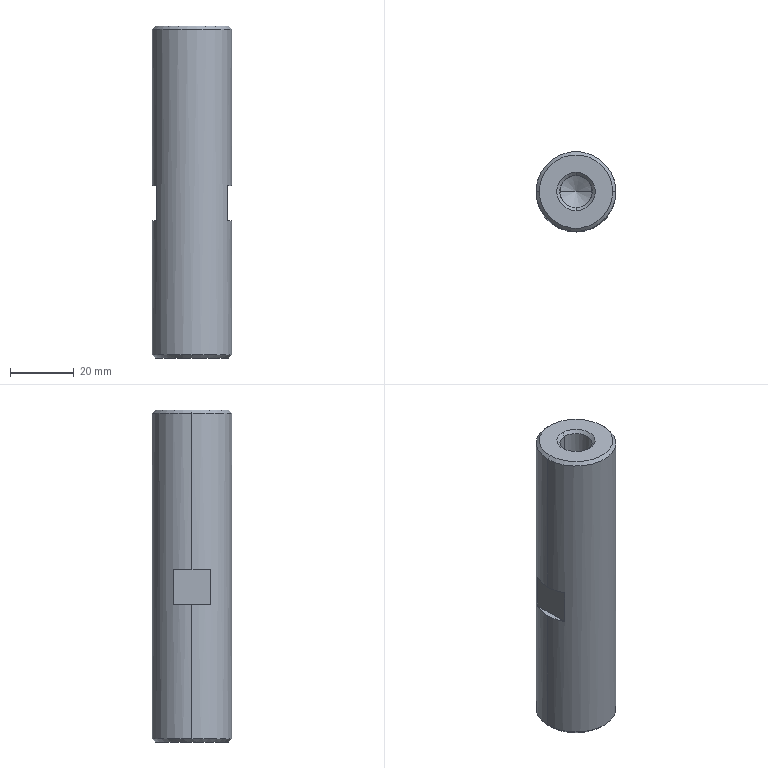Part | SolidWorks | features BaseBody 1, MoveFace 1 | 1 solid | 26 faces | box 25 x 25 x 104 mm | volume 46673 mm3 | cone 12 | plane 8 | cylinder 6 | commonest cylinder face diameters 10.106 x4 25 x2
STEP:
#1=CARTESIAN_POINT('',(0.,12.5,-103.));
#2=VERTEX_POINT('',#1);
#3=CARTESIAN_POINT('',(-12.5,0.,-103.));
#4=VERTEX_POINT('',#3);
#5=CARTESIAN_POINT('',(0.,0.,-103.));
#6=DIRECTION('',(0.,0.,1.));
#7=DIRECTION('',(1.,0.,0.));
#8=AXIS2_PLACEMENT_3D('',#5,#6,#7);
#9=CIRCLE('',#8,12.5);
#10=EDGE_CURVE('',#2,#4,#9,.T.);
#11=ORIENTED_EDGE('',*,*,#10,.T.);
#12=CARTESIAN_POINT('',(-12.5,0.,-61.));
#13=VERTEX_POINT('',#12);
#14=CARTESIAN_POINT('',(-12.5,0.,-106.));
#15=DIRECTION('',(0.,0.,1.));
#16=VECTOR('',#15,1000.);
#17=LINE('',#14,#16);
#18=EDGE_CURVE('',#4,#13,#17,.T.);
#19=ORIENTED_EDGE('',*,*,#18,.T.);
#20=CARTESIAN_POINT('',(-11.,5.937,-61.));
#21=VERTEX_POINT('',#20);
#22=CARTESIAN_POINT('',(0.,0.,-61.));
#23=DIRECTION('',(0.,0.,-1.));
#24=DIRECTION('',(1.,0.,0.));
#25=AXIS2_PLACEMENT_3D('',#22,#23,#24);
#26=CIRCLE('',#25,12.5);
#27=EDGE_CURVE('',#13,#21,#26,.T.);
#28=ORIENTED_EDGE('',*,*,#27,.T.);
#29=CARTESIAN_POINT('',(-11.,5.937,-50.));
#30=VERTEX_POINT('',#29);
#31=CARTESIAN_POINT('',(-11.,5.937,-106.));
#32=DIRECTION('',(0.,0.,1.));
#33=VECTOR('',#32,1000.);
#34=LINE('',#31,#33);
#35=EDGE_CURVE('',#21,#30,#34,.T.);
#36=ORIENTED_EDGE('',*,*,#35,.T.);
#37=CARTESIAN_POINT('',(-12.5,0.,-50.));
#38=VERTEX_POINT('',#37);
#39=CARTESIAN_POINT('',(0.,0.,-50.));
#40=DIRECTION('',(0.,0.,1.));
#41=DIRECTION('',(1.,0.,0.));
#42=AXIS2_PLACEMENT_3D('',#39,#40,#41);
#43=CIRCLE('',#42,12.5);
#44=EDGE_CURVE('',#30,#38,#43,.T.);
#45=ORIENTED_EDGE('',*,*,#44,.T.);
#46=CARTESIAN_POINT('',(-12.5,0.,-1.));
#47=VERTEX_POINT('',#46);
#48=CARTESIAN_POINT('',(-12.5,0.,-106.));
#49=DIRECTION('',(0.,0.,1.));
#50=VECTOR('',#49,1000.);
#51=LINE('',#48,#50);
#52=EDGE_CURVE('',#38,#47,#51,.T.);
#53=ORIENTED_EDGE('',*,*,#52,.T.);
#54=CARTESIAN_POINT('',(12.5,0.,-1.));
#55=VERTEX_POINT('',#54);
#56=CARTESIAN_POINT('',(0.,0.,-1.));
#57=DIRECTION('',(0.,0.,-1.));
#58=DIRECTION('',(1.,0.,0.));
#59=AXIS2_PLACEMENT_3D('',#56,#57,#58);
#60=CIRCLE('',#59,12.5);
#61=EDGE_CURVE('',#47,#55,#60,.T.);
#62=ORIENTED_EDGE('',*,*,#61,.T.);
#63=CARTESIAN_POINT('',(12.5,0.,-50.));
#64=VERTEX_POINT('',#63);
#65=CARTESIAN_POINT('',(12.5,0.,-106.));
#66=DIRECTION('',(0.,0.,1.));
#67=VECTOR('',#66,1000.);
#68=LINE('',#65,#67);
#69=EDGE_CURVE('',#64,#55,#68,.T.);
#70=ORIENTED_EDGE('',*,*,#69,.F.);
#71=CARTESIAN_POINT('',(11.,5.937,-50.));
#72=VERTEX_POINT('',#71);
#73=CARTESIAN_POINT('',(0.,0.,-50.));
#74=DIRECTION('',(0.,0.,1.));
#75=DIRECTION('',(1.,0.,0.));
#76=AXIS2_PLACEMENT_3D('',#73,#74,#75);
#77=CIRCLE('',#76,12.5);
#78=EDGE_CURVE('',#64,#72,#77,.T.);
#79=ORIENTED_EDGE('',*,*,#78,.T.);
#80=CARTESIAN_POINT('',(11.,5.937,-61.));
#81=VERTEX_POINT('',#80);
#82=CARTESIAN_POINT('',(11.,5.937,-106.));
#83=DIRECTION('',(0.,0.,-1.));
#84=VECTOR('',#83,1000.);
#85=LINE('',#82,#84);
#86=EDGE_CURVE('',#72,#81,#85,.T.);
#87=ORIENTED_EDGE('',*,*,#86,.T.);
#88=CARTESIAN_POINT('',(12.5,0.,-61.));
#89=VERTEX_POINT('',#88);
#90=CARTESIAN_POINT('',(0.,0.,-61.));
#91=DIRECTION('',(0.,0.,-1.));
#92=DIRECTION('',(1.,0.,0.));
#93=AXIS2_PLACEMENT_3D('',#90,#91,#92);
#94=CIRCLE('',#93,12.5);
#95=EDGE_CURVE('',#81,#89,#94,.T.);
#96=ORIENTED_EDGE('',*,*,#95,.T.);
#97=CARTESIAN_POINT('',(12.5,0.,-103.));
#98=VERTEX_POINT('',#97);
#99=CARTESIAN_POINT('',(12.5,0.,-106.));
#100=DIRECTION('',(0.,0.,1.));
#101=VECTOR('',#100,1000.);
#102=LINE('',#99,#101);
#103=EDGE_CURVE('',#98,#89,#102,.T.);
#104=ORIENTED_EDGE('',*,*,#103,.F.);
#105=CARTESIAN_POINT('',(0.,0.,-103.));
#106=DIRECTION('',(0.,0.,1.));
#107=DIRECTION('',(1.,0.,0.));
#108=AXIS2_PLACEMENT_3D('',#105,#106,#107);
#109=CIRCLE('',#108,12.5);
#110=EDGE_CURVE('',#98,#2,#109,.T.);
#111=ORIENTED_EDGE('',*,*,#110,.T.);
#112=EDGE_LOOP('',(#11,#19,#28,#36,#45,#53,#62,#70,#79,#87,#96,#104,#111));
#113=FACE_OUTER_BOUND('',#112,.T.);
#114=CARTESIAN_POINT('',(0.,0.,-106.));
#115=DIRECTION('',(0.,0.,1.));
#116=DIRECTION('',(1.,0.,0.));
#117=AXIS2_PLACEMENT_3D('',#114,#115,#116);
#118=CYLINDRICAL_SURFACE('',#117,12.5);
#119=ADVANCED_FACE('',(#113),#118,.T.);
#120=CARTESIAN_POINT('',(-11.5,0.,0.));
#121=VERTEX_POINT('',#120);
#122=CARTESIAN_POINT('',(11.5,0.,0.));
#123=VERTEX_POINT('',#122);
#124=CARTESIAN_POINT('',(0.,0.,0.));
#125=DIRECTION('',(0.,0.,-1.));
#126=DIRECTION('',(-1.,0.,0.));
#127=AXIS2_PLACEMENT_3D('',#124,#125,#126);
#128=CIRCLE('',#127,11.5);
#129=EDGE_CURVE('',#121,#123,#128,.T.);
#130=ORIENTED_EDGE('',*,*,#129,.T.);
#131=CARTESIAN_POINT('',(12.5,0.,-1.));
#132=DIRECTION('',(0.7071,0.,-0.7071));
#133=VECTOR('',#132,1000.);
#134=LINE('',#131,#133);
#135=EDGE_CURVE('',#123,#55,#134,.T.);
#136=ORIENTED_EDGE('',*,*,#135,.T.);
#137=ORIENTED_EDGE('',*,*,#61,.F.);
#138=CARTESIAN_POINT('',(-12.5,0.,-1.));
#139=DIRECTION('',(-0.7071,0.,-0.7071));
#140=VECTOR('',#139,1000.);
#141=LINE('',#138,#140);
#142=EDGE_CURVE('',#121,#47,#141,.T.);
#143=ORIENTED_EDGE('',*,*,#142,.F.);
#144=EDGE_LOOP('',(#130,#136,#137,#143));
#145=FACE_OUTER_BOUND('',#144,.T.);
#146=CARTESIAN_POINT('',(0.,0.,-1.));
#147=DIRECTION('',(0.,0.,-1.));
#148=DIRECTION('',(-1.,0.,0.));
#149=AXIS2_PLACEMENT_3D('',#146,#147,#148);
#150=CONICAL_SURFACE('',#149,12.5,0.7854);
#151=ADVANCED_FACE('',(#145),#150,.T.);
#152=CARTESIAN_POINT('',(0.,-11.5,-104.));
#153=VERTEX_POINT('',#152);
#154=CARTESIAN_POINT('',(0.,11.5,-104.));
#155=VERTEX_POINT('',#154);
#156=CARTESIAN_POINT('',(0.,0.,-104.));
#157=DIRECTION('',(0.,0.,1.));
#158=DIRECTION('',(0.,-1.,0.));
#159=AXIS2_PLACEMENT_3D('',#156,#157,#158);
#160=CIRCLE('',#159,11.5);
#161=EDGE_CURVE('',#153,#155,#160,.T.);
#162=ORIENTED_EDGE('',*,*,#161,.T.);
#163=CARTESIAN_POINT('',(0.,12.5,-103.));
#164=DIRECTION('',(0.,0.7071,0.7071));
#165=VECTOR('',#164,1000.);
#166=LINE('',#163,#165);
#167=EDGE_CURVE('',#155,#2,#166,.T.);
#168=ORIENTED_EDGE('',*,*,#167,.T.);
#169=ORIENTED_EDGE('',*,*,#110,.F.);
#170=CARTESIAN_POINT('',(0.,-12.5,-103.));
#171=VERTEX_POINT('',#170);
#172=CARTESIAN_POINT('',(0.,0.,-103.));
#173=DIRECTION('',(0.,0.,1.));
#174=DIRECTION('',(1.,0.,0.));
#175=AXIS2_PLACEMENT_3D('',#172,#173,#174);
#176=CIRCLE('',#175,12.5);
#177=EDGE_CURVE('',#171,#98,#176,.T.);
#178=ORIENTED_EDGE('',*,*,#177,.F.);
#179=CARTESIAN_POINT('',(0.,-12.5,-103.));
#180=DIRECTION('',(0.,-0.7071,0.7071));
#181=VECTOR('',#180,1000.);
#182=LINE('',#179,#181);
#183=EDGE_CURVE('',#153,#171,#182,.T.);
#184=ORIENTED_EDGE('',*,*,#183,.F.);
#185=EDGE_LOOP('',(#162,#168,#169,#178,#184));
#186=FACE_OUTER_BOUND('',#185,.T.);
#187=CARTESIAN_POINT('',(0.,0.,-103.));
#188=DIRECTION('',(0.,0.,1.));
#189=DIRECTION('',(0.,-1.,0.));
#190=AXIS2_PLACEMENT_3D('',#187,#188,#189);
#191=CONICAL_SURFACE('',#190,12.5,0.7854);
#192=ADVANCED_FACE('',(#186),#191,.T.);
#193=CARTESIAN_POINT('',(0.,5.053,-0.947));
#194=VERTEX_POINT('',#193);
#195=CARTESIAN_POINT('',(0.,-5.053,-0.947));
#196=VERTEX_POINT('',#195);
#197=CARTESIAN_POINT('',(0.,0.,-0.947));
#198=DIRECTION('',(0.,0.,1.));
#199=DIRECTION('',(0.,-1.,0.));
#200=AXIS2_PLACEMENT_3D('',#197,#198,#199);
#201=CIRCLE('',#200,5.053);
#202=EDGE_CURVE('',#194,#196,#201,.T.);
#203=ORIENTED_EDGE('',*,*,#202,.F.);
#204=CARTESIAN_POINT('',(0.,6.,0.));
#205=VERTEX_POINT('',#204);
#206=CARTESIAN_POINT('',(0.,6.,0.));
#207=DIRECTION('',(0.,0.7071,0.7071));
#208=VECTOR('',#207,1000.);
#209=LINE('',#206,#208);
#210=EDGE_CURVE('',#194,#205,#209,.T.);
#211=ORIENTED_EDGE('',*,*,#210,.T.);
#212=CARTESIAN_POINT('',(0.,-6.,0.));
#213=VERTEX_POINT('',#212);
#214=CARTESIAN_POINT('',(0.,0.,0.));
#215=DIRECTION('',(0.,0.,1.));
#216=DIRECTION('',(0.,-1.,0.));
#217=AXIS2_PLACEMENT_3D('',#214,#215,#216);
#218=CIRCLE('',#217,6.);
#219=EDGE_CURVE('',#205,#213,#218,.T.);
#220=ORIENTED_EDGE('',*,*,#219,.T.);
#221=CARTESIAN_POINT('',(0.,-6.,0.));
#222=DIRECTION('',(0.,-0.7071,0.7071));
#223=VECTOR('',#222,1000.);
#224=LINE('',#221,#223);
#225=EDGE_CURVE('',#196,#213,#224,.T.);
#226=ORIENTED_EDGE('',*,*,#225,.F.);
#227=EDGE_LOOP('',(#203,#211,#220,#226));
#228=FACE_OUTER_BOUND('',#227,.T.);
#229=CARTESIAN_POINT('',(0.,0.,0.));
#230=DIRECTION('',(0.,0.,1.));
#231=DIRECTION('',(0.,-1.,0.));
#232=AXIS2_PLACEMENT_3D('',#229,#230,#231);
#233=CONICAL_SURFACE('',#232,6.,0.7854);
#234=ADVANCED_FACE('',(#228),#233,.F.);
#235=CARTESIAN_POINT('',(0.,-5.053,-103.053));
#236=VERTEX_POINT('',#235);
#237=CARTESIAN_POINT('',(-5.053,0.,-103.053));
#238=VERTEX_POINT('',#237);
#239=CARTESIAN_POINT('',(0.,0.,-103.053));
#240=DIRECTION('',(0.,0.,-1.));
#241=DIRECTION('',(-1.,0.,0.));
#242=AXIS2_PLACEMENT_3D('',#239,#240,#241);
#243=CIRCLE('',#242,5.053);
#244=EDGE_CURVE('',#236,#238,#243,.T.);
#245=ORIENTED_EDGE('',*,*,#244,.F.);
#246=CARTESIAN_POINT('',(0.,-6.,-104.));
#247=VERTEX_POINT('',#246);
#248=CARTESIAN_POINT('',(0.,-6.,-104.));
#249=DIRECTION('',(0.,-0.7071,-0.7071));
#250=VECTOR('',#249,1000.);
#251=LINE('',#248,#250);
#252=EDGE_CURVE('',#236,#247,#251,.T.);
#253=ORIENTED_EDGE('',*,*,#252,.T.);
#254=CARTESIAN_POINT('',(0.,6.,-104.));
#255=VERTEX_POINT('',#254);
#256=CARTESIAN_POINT('',(0.,0.,-104.));
#257=DIRECTION('',(0.,0.,-1.));
#258=DIRECTION('',(0.,1.,0.));
#259=AXIS2_PLACEMENT_3D('',#256,#257,#258);
#260=CIRCLE('',#259,6.);
#261=EDGE_CURVE('',#247,#255,#260,.T.);
#262=ORIENTED_EDGE('',*,*,#261,.T.);
#263=CARTESIAN_POINT('',(0.,5.053,-103.053));
#264=VERTEX_POINT('',#263);
#265=CARTESIAN_POINT('',(0.,6.,-104.));
#266=DIRECTION('',(0.,0.7071,-0.7071));
#267=VECTOR('',#266,1000.);
#268=LINE('',#265,#267);
#269=EDGE_CURVE('',#264,#255,#268,.T.);
#270=ORIENTED_EDGE('',*,*,#269,.F.);
#271=CARTESIAN_POINT('',(0.,0.,-103.053));
#272=DIRECTION('',(0.,0.,-1.));
#273=DIRECTION('',(-1.,0.,0.));
#274=AXIS2_PLACEMENT_3D('',#271,#272,#273);
#275=CIRCLE('',#274,5.053);
#276=EDGE_CURVE('',#238,#264,#275,.T.);
#277=ORIENTED_EDGE('',*,*,#276,.F.);
#278=EDGE_LOOP('',(#245,#253,#262,#270,#277));
#279=FACE_OUTER_BOUND('',#278,.T.);
#280=CARTESIAN_POINT('',(0.,0.,-104.));
#281=DIRECTION('',(0.,0.,-1.));
#282=DIRECTION('',(0.,1.,0.));
#283=AXIS2_PLACEMENT_3D('',#280,#281,#282);
#284=CONICAL_SURFACE('',#283,6.,0.7854);
#285=ADVANCED_FACE('',(#279),#284,.F.);
#286=CARTESIAN_POINT('',(0.,5.053,-24.));
#287=VERTEX_POINT('',#286);
#288=CARTESIAN_POINT('',(-5.053,0.,-24.));
#289=VERTEX_POINT('',#288);
#290=CARTESIAN_POINT('',(0.,0.,-24.));
#291=DIRECTION('',(0.,0.,1.));
#292=DIRECTION('',(0.,-1.,0.));
#293=AXIS2_PLACEMENT_3D('',#290,#291,#292);
#294=CIRCLE('',#293,5.053);
#295=EDGE_CURVE('',#287,#289,#294,.T.);
#296=ORIENTED_EDGE('',*,*,#295,.F.);
#297=CARTESIAN_POINT('',(0.,5.053,-26.917));
#298=DIRECTION('',(0.,0.,1.));
#299=VECTOR('',#298,1000.);
#300=LINE('',#297,#299);
#301=EDGE_CURVE('',#287,#194,#300,.T.);
#302=ORIENTED_EDGE('',*,*,#301,.T.);
#303=ORIENTED_EDGE('',*,*,#202,.T.);
#304=CARTESIAN_POINT('',(0.,-5.053,-24.));
#305=VERTEX_POINT('',#304);
#306=CARTESIAN_POINT('',(0.,-5.053,-26.917));
#307=DIRECTION('',(0.,0.,1.));
#308=VECTOR('',#307,1000.);
#309=LINE('',#306,#308);
#310=EDGE_CURVE('',#305,#196,#309,.T.);
#311=ORIENTED_EDGE('',*,*,#310,.F.);
#312=CARTESIAN_POINT('',(0.,0.,-24.));
#313=DIRECTION('',(0.,0.,1.));
#314=DIRECTION('',(0.,-1.,0.));
#315=AXIS2_PLACEMENT_3D('',#312,#313,#314);
#316=CIRCLE('',#315,5.053);
#317=EDGE_CURVE('',#289,#305,#316,.T.);
#318=ORIENTED_EDGE('',*,*,#317,.F.);
#319=EDGE_LOOP('',(#296,#302,#303,#311,#318));
#320=FACE_OUTER_BOUND('',#319,.T.);
#321=CARTESIAN_POINT('',(0.,0.,-26.917));
#322=DIRECTION('',(0.,0.,1.));
#323=DIRECTION('',(0.,-1.,0.));
#324=AXIS2_PLACEMENT_3D('',#321,#322,#323);
#325=CYLINDRICAL_SURFACE('',#324,5.053);
#326=ADVANCED_FACE('',(#320),#325,.F.);
#327=CARTESIAN_POINT('',(5.053,0.,-103.053));
#328=VERTEX_POINT('',#327);
#329=CARTESIAN_POINT('',(0.,0.,-103.053));
#330=DIRECTION('',(0.,0.,-1.));
#331=DIRECTION('',(-1.,0.,0.));
#332=AXIS2_PLACEMENT_3D('',#329,#330,#331);
#333=CIRCLE('',#332,5.053);
#334=EDGE_CURVE('',#328,#236,#333,.T.);
#335=ORIENTED_EDGE('',*,*,#334,.T.);
#336=ORIENTED_EDGE('',*,*,#244,.T.);
#337=CARTESIAN_POINT('',(-5.053,0.,-80.));
#338=VERTEX_POINT('',#337);
#339=CARTESIAN_POINT('',(-5.053,0.,-104.));
#340=DIRECTION('',(0.,0.,1.));
#341=VECTOR('',#340,1000.);
#342=LINE('',#339,#341);
#343=EDGE_CURVE('',#238,#338,#342,.T.);
#344=ORIENTED_EDGE('',*,*,#343,.T.);
#345=CARTESIAN_POINT('',(5.053,0.,-80.));
#346=VERTEX_POINT('',#345);
#347=CARTESIAN_POINT('',(0.,0.,-80.));
#348=DIRECTION('',(0.,0.,-1.));
#349=DIRECTION('',(1.,0.,0.));
#350=AXIS2_PLACEMENT_3D('',#347,#348,#349);
#351=CIRCLE('',#350,5.053);
#352=EDGE_CURVE('',#346,#338,#351,.T.);
#353=ORIENTED_EDGE('',*,*,#352,.F.);
#354=CARTESIAN_POINT('',(5.053,0.,-104.));
#355=DIRECTION('',(0.,0.,1.));
#356=VECTOR('',#355,1000.);
#357=LINE('',#354,#356);
#358=EDGE_CURVE('',#328,#346,#357,.T.);
#359=ORIENTED_EDGE('',*,*,#358,.F.);
#360=EDGE_LOOP('',(#335,#336,#344,#353,#359));
#361=FACE_OUTER_BOUND('',#360,.T.);
#362=CARTESIAN_POINT('',(0.,0.,-104.));
#363=DIRECTION('',(0.,0.,1.));
#364=DIRECTION('',(1.,0.,0.));
#365=AXIS2_PLACEMENT_3D('',#362,#363,#364);
#366=CYLINDRICAL_SURFACE('',#365,5.053);
#367=ADVANCED_FACE('',(#361),#366,.F.);
#368=CARTESIAN_POINT('',(0.,0.,-26.917));
#369=VERTEX_POINT('',#368);
#370=CARTESIAN_POINT('',(5.053,0.,-24.));
#371=VERTEX_POINT('',#370);
#372=CARTESIAN_POINT('',(5.053,0.,-24.));
#373=DIRECTION('',(0.866,0.,0.5));
#374=VECTOR('',#373,1000.);
#375=LINE('',#372,#374);
#376=EDGE_CURVE('',#369,#371,#375,.T.);
#377=ORIENTED_EDGE('',*,*,#376,.F.);
#378=CARTESIAN_POINT('',(-5.053,0.,-24.));
#379=DIRECTION('',(-0.866,0.,0.5));
#380=VECTOR('',#379,1000.);
#381=LINE('',#378,#380);
#382=EDGE_CURVE('',#369,#289,#381,.T.);
#383=ORIENTED_EDGE('',*,*,#382,.T.);
#384=ORIENTED_EDGE('',*,*,#317,.T.);
#385=CARTESIAN_POINT('',(0.,0.,-24.));
#386=DIRECTION('',(0.,0.,1.));
#387=DIRECTION('',(0.,-1.,0.));
#388=AXIS2_PLACEMENT_3D('',#385,#386,#387);
#389=CIRCLE('',#388,5.053);
#390=EDGE_CURVE('',#305,#371,#389,.T.);
#391=ORIENTED_EDGE('',*,*,#390,.T.);
#392=EDGE_LOOP('',(#377,#383,#384,#391));
#393=FACE_OUTER_BOUND('',#392,.T.);
#394=CARTESIAN_POINT('',(0.,0.,-24.));
#395=DIRECTION('',(0.,0.,1.));
#396=DIRECTION('',(1.,0.,0.));
#397=AXIS2_PLACEMENT_3D('',#394,#395,#396);
#398=CONICAL_SURFACE('',#397,5.053,1.047);
#399=ADVANCED_FACE('',(#393),#398,.F.);
#400=CARTESIAN_POINT('',(0.,0.,-77.083));
#401=VERTEX_POINT('',#400);
#402=CARTESIAN_POINT('',(-5.053,0.,-80.));
#403=DIRECTION('',(-0.866,0.,-0.5));
#404=VECTOR('',#403,1000.);
#405=LINE('',#402,#404);
#406=EDGE_CURVE('',#401,#338,#405,.T.);
#407=ORIENTED_EDGE('',*,*,#406,.F.);
#408=CARTESIAN_POINT('',(5.053,0.,-80.));
#409=DIRECTION('',(0.866,0.,-0.5));
#410=VECTOR('',#409,1000.);
#411=LINE('',#408,#410);
#412=EDGE_CURVE('',#401,#346,#411,.T.);
#413=ORIENTED_EDGE('',*,*,#412,.T.);
#414=ORIENTED_EDGE('',*,*,#352,.T.);
#415=EDGE_LOOP('',(#407,#413,#414));
#416=FACE_OUTER_BOUND('',#415,.T.);
#417=CARTESIAN_POINT('',(0.,0.,-80.));
#418=DIRECTION('',(0.,0.,-1.));
#419=DIRECTION('',(-1.,0.,0.));
#420=AXIS2_PLACEMENT_3D('',#417,#418,#419);
#421=CONICAL_SURFACE('',#420,5.053,1.047);
#422=ADVANCED_FACE('',(#416),#421,.F.);
#423=ORIENTED_EDGE('',*,*,#18,.F.);
#424=CARTESIAN_POINT('',(0.,0.,-103.));
#425=DIRECTION('',(0.,0.,1.));
#426=DIRECTION('',(1.,0.,0.));
#427=AXIS2_PLACEMENT_3D('',#424,#425,#426);
#428=CIRCLE('',#427,12.5);
#429=EDGE_CURVE('',#4,#171,#428,.T.);
#430=ORIENTED_EDGE('',*,*,#429,.T.);
#431=ORIENTED_EDGE('',*,*,#177,.T.);
#432=ORIENTED_EDGE('',*,*,#103,.T.);
#433=CARTESIAN_POINT('',(11.,-5.937,-61.));
#434=VERTEX_POINT('',#433);
#435=CARTESIAN_POINT('',(0.,0.,-61.));
#436=DIRECTION('',(0.,0.,-1.));
#437=DIRECTION('',(1.,0.,0.));
#438=AXIS2_PLACEMENT_3D('',#435,#436,#437);
#439=CIRCLE('',#438,12.5);
#440=EDGE_CURVE('',#89,#434,#439,.T.);
#441=ORIENTED_EDGE('',*,*,#440,.T.);
#442=CARTESIAN_POINT('',(11.,-5.937,-50.));
#443=VERTEX_POINT('',#442);
#444=CARTESIAN_POINT('',(11.,-5.937,-106.));
#445=DIRECTION('',(0.,0.,1.));
#446=VECTOR('',#445,1000.);
#447=LINE('',#444,#446);
#448=EDGE_CURVE('',#434,#443,#447,.T.);
#449=ORIENTED_EDGE('',*,*,#448,.T.);
#450=CARTESIAN_POINT('',(0.,0.,-50.));
#451=DIRECTION('',(0.,0.,1.));
#452=DIRECTION('',(1.,0.,0.));
#453=AXIS2_PLACEMENT_3D('',#450,#451,#452);
#454=CIRCLE('',#453,12.5);
#455=EDGE_CURVE('',#443,#64,#454,.T.);
#456=ORIENTED_EDGE('',*,*,#455,.T.);
#457=ORIENTED_EDGE('',*,*,#69,.T.);
#458=CARTESIAN_POINT('',(0.,0.,-1.));
#459=DIRECTION('',(0.,0.,-1.));
#460=DIRECTION('',(1.,0.,0.));
#461=AXIS2_PLACEMENT_3D('',#458,#459,#460);
#462=CIRCLE('',#461,12.5);
#463=EDGE_CURVE('',#55,#47,#462,.T.);
#464=ORIENTED_EDGE('',*,*,#463,.T.);
#465=ORIENTED_EDGE('',*,*,#52,.F.);
#466=CARTESIAN_POINT('',(-11.,-5.937,-50.));
#467=VERTEX_POINT('',#466);
#468=CARTESIAN_POINT('',(0.,0.,-50.));
#469=DIRECTION('',(0.,0.,1.));
#470=DIRECTION('',(1.,0.,0.));
#471=AXIS2_PLACEMENT_3D('',#468,#469,#470);
#472=CIRCLE('',#471,12.5);
#473=EDGE_CURVE('',#38,#467,#472,.T.);
#474=ORIENTED_EDGE('',*,*,#473,.T.);
#475=CARTESIAN_POINT('',(-11.,-5.937,-61.));
#476=VERTEX_POINT('',#475);
#477=CARTESIAN_POINT('',(-11.,-5.937,-106.));
#478=DIRECTION('',(0.,0.,-1.));
#479=VECTOR('',#478,1000.);
#480=LINE('',#477,#479);
#481=EDGE_CURVE('',#467,#476,#480,.T.);
#482=ORIENTED_EDGE('',*,*,#481,.T.);
#483=CARTESIAN_POINT('',(0.,0.,-61.));
#484=DIRECTION('',(0.,0.,-1.));
#485=DIRECTION('',(1.,0.,0.));
#486=AXIS2_PLACEMENT_3D('',#483,#484,#485);
#487=CIRCLE('',#486,12.5);
#488=EDGE_CURVE('',#476,#13,#487,.T.);
#489=ORIENTED_EDGE('',*,*,#488,.T.);
#490=EDGE_LOOP('',(#423,#430,#431,#432,#441,#449,#456,#457,#464,#465,#474,#482,#489));
#491=FACE_OUTER_BOUND('',#490,.T.);
#492=CARTESIAN_POINT('',(0.,0.,-106.));
#493=DIRECTION('',(0.,0.,1.));
#494=DIRECTION('',(1.,0.,0.));
#495=AXIS2_PLACEMENT_3D('',#492,#493,#494);
#496=CYLINDRICAL_SURFACE('',#495,12.5);
#497=ADVANCED_FACE('',(#491),#496,.T.);
#498=CARTESIAN_POINT('',(11.,-5.937,-61.));
#499=DIRECTION('',(0.,1.,0.));
#500=VECTOR('',#499,1000.);
#501=LINE('',#498,#500);
#502=EDGE_CURVE('',#434,#81,#501,.T.);
#503=ORIENTED_EDGE('',*,*,#502,.T.);
#504=ORIENTED_EDGE('',*,*,#86,.F.);
#505=CARTESIAN_POINT('',(11.,-5.937,-50.));
#506=DIRECTION('',(0.,-1.,0.));
#507=VECTOR('',#506,1000.);
#508=LINE('',#505,#507);
#509=EDGE_CURVE('',#72,#443,#508,.T.);
#510=ORIENTED_EDGE('',*,*,#509,.T.);
#511=ORIENTED_EDGE('',*,*,#448,.F.);
#512=EDGE_LOOP('',(#503,#504,#510,#511));
#513=FACE_OUTER_BOUND('',#512,.T.);
#514=CARTESIAN_POINT('',(11.,-5.937,-61.));
#515=DIRECTION('',(1.,0.,0.));
#516=DIRECTION('',(0.,0.,-1.));
#517=AXIS2_PLACEMENT_3D('',#514,#515,#516);
#518=PLANE('',#517);
#519=ADVANCED_FACE('',(#513),#518,.T.);
#520=ORIENTED_EDGE('',*,*,#95,.F.);
#521=ORIENTED_EDGE('',*,*,#502,.F.);
#522=ORIENTED_EDGE('',*,*,#440,.F.);
#523=EDGE_LOOP('',(#520,#521,#522));
#524=FACE_OUTER_BOUND('',#523,.T.);
#525=CARTESIAN_POINT('',(0.,0.,-61.));
#526=DIRECTION('',(0.,0.,1.));
#527=DIRECTION('',(1.,0.,0.));
#528=AXIS2_PLACEMENT_3D('',#525,#526,#527);
#529=PLANE('',#528);
#530=ADVANCED_FACE('',(#524),#529,.T.);
#531=ORIENTED_EDGE('',*,*,#455,.F.);
#532=ORIENTED_EDGE('',*,*,#509,.F.);
#533=ORIENTED_EDGE('',*,*,#78,.F.);
#534=EDGE_LOOP('',(#531,#532,#533));
#535=FACE_OUTER_BOUND('',#534,.T.);
#536=CARTESIAN_POINT('',(0.,0.,-50.));
#537=DIRECTION('',(0.,0.,1.));
#538=DIRECTION('',(1.,0.,0.));
#539=AXIS2_PLACEMENT_3D('',#536,#537,#538);
#540=PLANE('',#539);
#541=ADVANCED_FACE('',(#535),#540,.F.);
#542=CARTESIAN_POINT('',(-11.,5.937,-61.));
#543=DIRECTION('',(0.,-1.,0.));
#544=VECTOR('',#543,1000.);
#545=LINE('',#542,#544);
#546=EDGE_CURVE('',#21,#476,#545,.T.);
#547=ORIENTED_EDGE('',*,*,#546,.T.);
#548=ORIENTED_EDGE('',*,*,#481,.F.);
#549=CARTESIAN_POINT('',(-11.,5.937,-50.));
#550=DIRECTION('',(0.,1.,0.));
#551=VECTOR('',#550,1000.);
#552=LINE('',#549,#551);
#553=EDGE_CURVE('',#467,#30,#552,.T.);
#554=ORIENTED_EDGE('',*,*,#553,.T.);
#555=ORIENTED_EDGE('',*,*,#35,.F.);
#556=EDGE_LOOP('',(#547,#548,#554,#555));
#557=FACE_OUTER_BOUND('',#556,.T.);
#558=CARTESIAN_POINT('',(-11.,5.937,-61.));
#559=DIRECTION('',(-1.,0.,0.));
#560=DIRECTION('',(0.,0.,1.));
#561=AXIS2_PLACEMENT_3D('',#558,#559,#560);
#562=PLANE('',#561);
#563=ADVANCED_FACE('',(#557),#562,.T.);
#564=ORIENTED_EDGE('',*,*,#44,.F.);
#565=ORIENTED_EDGE('',*,*,#553,.F.);
#566=ORIENTED_EDGE('',*,*,#473,.F.);
#567=EDGE_LOOP('',(#564,#565,#566));
#568=FACE_OUTER_BOUND('',#567,.T.);
#569=CARTESIAN_POINT('',(0.,0.,-50.));
#570=DIRECTION('',(0.,0.,1.));
#571=DIRECTION('',(1.,0.,0.));
#572=AXIS2_PLACEMENT_3D('',#569,#570,#571);
#573=PLANE('',#572);
#574=ADVANCED_FACE('',(#568),#573,.F.);
#575=ORIENTED_EDGE('',*,*,#488,.F.);
#576=ORIENTED_EDGE('',*,*,#546,.F.);
#577=ORIENTED_EDGE('',*,*,#27,.F.);
#578=EDGE_LOOP('',(#575,#576,#577));
#579=FACE_OUTER_BOUND('',#578,.T.);
#580=CARTESIAN_POINT('',(0.,0.,-61.));
#581=DIRECTION('',(0.,0.,1.));
#582=DIRECTION('',(1.,0.,0.));
#583=AXIS2_PLACEMENT_3D('',#580,#581,#582);
#584=PLANE('',#583);
#585=ADVANCED_FACE('',(#579),#584,.T.);
#586=ORIENTED_EDGE('',*,*,#135,.F.);
#587=CARTESIAN_POINT('',(0.,0.,0.));
#588=DIRECTION('',(0.,0.,-1.));
#589=DIRECTION('',(-1.,0.,0.));
#590=AXIS2_PLACEMENT_3D('',#587,#588,#589);
#591=CIRCLE('',#590,11.5);
#592=EDGE_CURVE('',#123,#121,#591,.T.);
#593=ORIENTED_EDGE('',*,*,#592,.T.);
#594=ORIENTED_EDGE('',*,*,#142,.T.);
#595=ORIENTED_EDGE('',*,*,#463,.F.);
#596=EDGE_LOOP('',(#586,#593,#594,#595));
#597=FACE_OUTER_BOUND('',#596,.T.);
#598=CARTESIAN_POINT('',(0.,0.,-1.));
#599=DIRECTION('',(0.,0.,-1.));
#600=DIRECTION('',(-1.,0.,0.));
#601=AXIS2_PLACEMENT_3D('',#598,#599,#600);
#602=CONICAL_SURFACE('',#601,12.5,0.7854);
#603=ADVANCED_FACE('',(#597),#602,.T.);
#604=ORIENTED_EDGE('',*,*,#167,.F.);
#605=CARTESIAN_POINT('',(0.,0.,-104.));
#606=DIRECTION('',(0.,0.,1.));
#607=DIRECTION('',(0.,-1.,0.));
#608=AXIS2_PLACEMENT_3D('',#605,#606,#607);
#609=CIRCLE('',#608,11.5);
#610=EDGE_CURVE('',#155,#153,#609,.T.);
#611=ORIENTED_EDGE('',*,*,#610,.T.);
#612=ORIENTED_EDGE('',*,*,#183,.T.);
#613=ORIENTED_EDGE('',*,*,#429,.F.);
#614=ORIENTED_EDGE('',*,*,#10,.F.);
#615=EDGE_LOOP('',(#604,#611,#612,#613,#614));
#616=FACE_OUTER_BOUND('',#615,.T.);
#617=CARTESIAN_POINT('',(0.,0.,-103.));
#618=DIRECTION('',(0.,0.,1.));
#619=DIRECTION('',(0.,-1.,0.));
#620=AXIS2_PLACEMENT_3D('',#617,#618,#619);
#621=CONICAL_SURFACE('',#620,12.5,0.7854);
#622=ADVANCED_FACE('',(#616),#621,.T.);
#623=CARTESIAN_POINT('',(0.,0.,0.));
#624=DIRECTION('',(0.,0.,1.));
#625=DIRECTION('',(0.,-1.,0.));
#626=AXIS2_PLACEMENT_3D('',#623,#624,#625);
#627=CIRCLE('',#626,6.);
#628=EDGE_CURVE('',#213,#205,#627,.T.);
#629=ORIENTED_EDGE('',*,*,#628,.F.);
#630=ORIENTED_EDGE('',*,*,#219,.F.);
#631=EDGE_LOOP('',(#629,#630));
#632=FACE_BOUND('',#631,.T.);
#633=ORIENTED_EDGE('',*,*,#129,.F.);
#634=ORIENTED_EDGE('',*,*,#592,.F.);
#635=EDGE_LOOP('',(#633,#634));
#636=FACE_OUTER_BOUND('',#635,.T.);
#637=CARTESIAN_POINT('',(0.,0.,0.));
#638=DIRECTION('',(0.,0.,-1.));
#639=DIRECTION('',(-1.,0.,0.));
#640=AXIS2_PLACEMENT_3D('',#637,#638,#639);
#641=PLANE('',#640);
#642=ADVANCED_FACE('',(#632,#636),#641,.F.);
#643=ORIENTED_EDGE('',*,*,#161,.F.);
#644=ORIENTED_EDGE('',*,*,#610,.F.);
#645=EDGE_LOOP('',(#643,#644));
#646=FACE_OUTER_BOUND('',#645,.T.);
#647=CARTESIAN_POINT('',(0.,0.,-104.));
#648=DIRECTION('',(0.,0.,-1.));
#649=DIRECTION('',(0.,1.,0.));
#650=AXIS2_PLACEMENT_3D('',#647,#648,#649);
#651=CIRCLE('',#650,6.);
#652=EDGE_CURVE('',#255,#247,#651,.T.);
#653=ORIENTED_EDGE('',*,*,#652,.F.);
#654=ORIENTED_EDGE('',*,*,#261,.F.);
#655=EDGE_LOOP('',(#653,#654));
#656=FACE_BOUND('',#655,.T.);
#657=CARTESIAN_POINT('',(0.,11.5,-104.));
#658=DIRECTION('',(0.,0.,1.));
#659=DIRECTION('',(1.,0.,0.));
#660=AXIS2_PLACEMENT_3D('',#657,#658,#659);
#661=PLANE('',#660);
#662=ADVANCED_FACE('',(#646,#656),#661,.F.);
#663=ORIENTED_EDGE('',*,*,#210,.F.);
#664=CARTESIAN_POINT('',(0.,0.,-0.947));
#665=DIRECTION('',(0.,0.,1.));
#666=DIRECTION('',(0.,-1.,0.));
#667=AXIS2_PLACEMENT_3D('',#664,#665,#666);
#668=CIRCLE('',#667,5.053);
#669=EDGE_CURVE('',#196,#194,#668,.T.);
#670=ORIENTED_EDGE('',*,*,#669,.F.);
#671=ORIENTED_EDGE('',*,*,#225,.T.);
#672=ORIENTED_EDGE('',*,*,#628,.T.);
#673=EDGE_LOOP('',(#663,#670,#671,#672));
#674=FACE_OUTER_BOUND('',#673,.T.);
#675=CARTESIAN_POINT('',(0.,0.,0.));
#676=DIRECTION('',(0.,0.,1.));
#677=DIRECTION('',(0.,-1.,0.));
#678=AXIS2_PLACEMENT_3D('',#675,#676,#677);
#679=CONICAL_SURFACE('',#678,6.,0.7854);
#680=ADVANCED_FACE('',(#674),#679,.F.);
#681=ORIENTED_EDGE('',*,*,#252,.F.);
#682=ORIENTED_EDGE('',*,*,#334,.F.);
#683=CARTESIAN_POINT('',(0.,0.,-103.053));
#684=DIRECTION('',(0.,0.,-1.));
#685=DIRECTION('',(-1.,0.,0.));
#686=AXIS2_PLACEMENT_3D('',#683,#684,#685);
#687=CIRCLE('',#686,5.053);
#688=EDGE_CURVE('',#264,#328,#687,.T.);
#689=ORIENTED_EDGE('',*,*,#688,.F.);
#690=ORIENTED_EDGE('',*,*,#269,.T.);
#691=ORIENTED_EDGE('',*,*,#652,.T.);
#692=EDGE_LOOP('',(#681,#682,#689,#690,#691));
#693=FACE_OUTER_BOUND('',#692,.T.);
#694=CARTESIAN_POINT('',(0.,0.,-104.));
#695=DIRECTION('',(0.,0.,-1.));
#696=DIRECTION('',(0.,1.,0.));
#697=AXIS2_PLACEMENT_3D('',#694,#695,#696);
#698=CONICAL_SURFACE('',#697,6.,0.7854);
#699=ADVANCED_FACE('',(#693),#698,.F.);
#700=ORIENTED_EDGE('',*,*,#301,.F.);
#701=CARTESIAN_POINT('',(0.,0.,-24.));
#702=DIRECTION('',(0.,0.,1.));
#703=DIRECTION('',(0.,-1.,0.));
#704=AXIS2_PLACEMENT_3D('',#701,#702,#703);
#705=CIRCLE('',#704,5.053);
#706=EDGE_CURVE('',#371,#287,#705,.T.);
#707=ORIENTED_EDGE('',*,*,#706,.F.);
#708=ORIENTED_EDGE('',*,*,#390,.F.);
#709=ORIENTED_EDGE('',*,*,#310,.T.);
#710=ORIENTED_EDGE('',*,*,#669,.T.);
#711=EDGE_LOOP('',(#700,#707,#708,#709,#710));
#712=FACE_OUTER_BOUND('',#711,.T.);
#713=CARTESIAN_POINT('',(0.,0.,-26.917));
#714=DIRECTION('',(0.,0.,1.));
#715=DIRECTION('',(0.,-1.,0.));
#716=AXIS2_PLACEMENT_3D('',#713,#714,#715);
#717=CYLINDRICAL_SURFACE('',#716,5.053);
#718=ADVANCED_FACE('',(#712),#717,.F.);
#719=ORIENTED_EDGE('',*,*,#343,.F.);
#720=ORIENTED_EDGE('',*,*,#276,.T.);
#721=ORIENTED_EDGE('',*,*,#688,.T.);
#722=ORIENTED_EDGE('',*,*,#358,.T.);
#723=CARTESIAN_POINT('',(0.,0.,-80.));
#724=DIRECTION('',(0.,0.,-1.));
#725=DIRECTION('',(1.,0.,0.));
#726=AXIS2_PLACEMENT_3D('',#723,#724,#725);
#727=CIRCLE('',#726,5.053);
#728=EDGE_CURVE('',#338,#346,#727,.T.);
#729=ORIENTED_EDGE('',*,*,#728,.F.);
#730=EDGE_LOOP('',(#719,#720,#721,#722,#729));
#731=FACE_OUTER_BOUND('',#730,.T.);
#732=CARTESIAN_POINT('',(0.,0.,-104.));
#733=DIRECTION('',(0.,0.,1.));
#734=DIRECTION('',(1.,0.,0.));
#735=AXIS2_PLACEMENT_3D('',#732,#733,#734);
#736=CYLINDRICAL_SURFACE('',#735,5.053);
#737=ADVANCED_FACE('',(#731),#736,.F.);
#738=ORIENTED_EDGE('',*,*,#382,.F.);
#739=ORIENTED_EDGE('',*,*,#376,.T.);
#740=ORIENTED_EDGE('',*,*,#706,.T.);
#741=ORIENTED_EDGE('',*,*,#295,.T.);
#742=EDGE_LOOP('',(#738,#739,#740,#741));
#743=FACE_OUTER_BOUND('',#742,.T.);
#744=CARTESIAN_POINT('',(0.,0.,-24.));
#745=DIRECTION('',(0.,0.,1.));
#746=DIRECTION('',(1.,0.,0.));
#747=AXIS2_PLACEMENT_3D('',#744,#745,#746);
#748=CONICAL_SURFACE('',#747,5.053,1.047);
#749=ADVANCED_FACE('',(#743),#748,.F.);
#750=ORIENTED_EDGE('',*,*,#412,.F.);
#751=ORIENTED_EDGE('',*,*,#406,.T.);
#752=ORIENTED_EDGE('',*,*,#728,.T.);
#753=EDGE_LOOP('',(#750,#751,#752));
#754=FACE_OUTER_BOUND('',#753,.T.);
#755=CARTESIAN_POINT('',(0.,0.,-80.));
#756=DIRECTION('',(0.,0.,-1.));
#757=DIRECTION('',(-1.,0.,0.));
#758=AXIS2_PLACEMENT_3D('',#755,#756,#757);
#759=CONICAL_SURFACE('',#758,5.053,1.047);
#760=ADVANCED_FACE('',(#754),#759,.F.);
#761=CLOSED_SHELL('',(#119,#151,#192,#234,#285,#326,#367,#399,#422,#497,#519,#530,#541,#563,#574,#585,#603,#622,#642,#662,#680,#699,#718,#737,#749,#760));
#762=MANIFOLD_SOLID_BREP('',#761);
#763=CARTESIAN_POINT('',(0.,0.,0.));
#764=DIRECTION('',(0.,0.,1.));
#765=DIRECTION('',(1.,0.,0.));
#766=AXIS2_PLACEMENT_3D('',#763,#764,#765);
#767=(LENGTH_UNIT()NAMED_UNIT(*)SI_UNIT(.MILLI.,.METRE.));
#768=UNCERTAINTY_MEASURE_WITH_UNIT(LENGTH_MEASURE(0.00001),#767,'','');
#769=(NAMED_UNIT(*)PLANE_ANGLE_UNIT()SI_UNIT($,.RADIAN.));
#770=(NAMED_UNIT(*)SI_UNIT($,.STERADIAN.)SOLID_ANGLE_UNIT());
#771=(GEOMETRIC_REPRESENTATION_CONTEXT(3)GLOBAL_UNCERTAINTY_ASSIGNED_CONTEXT((#768))GLOBAL_UNIT_ASSIGNED_CONTEXT((#767,#769,#770))REPRESENTATION_CONTEXT('',''));
#772=ADVANCED_BREP_SHAPE_REPRESENTATION('',(#762,#766),#771);